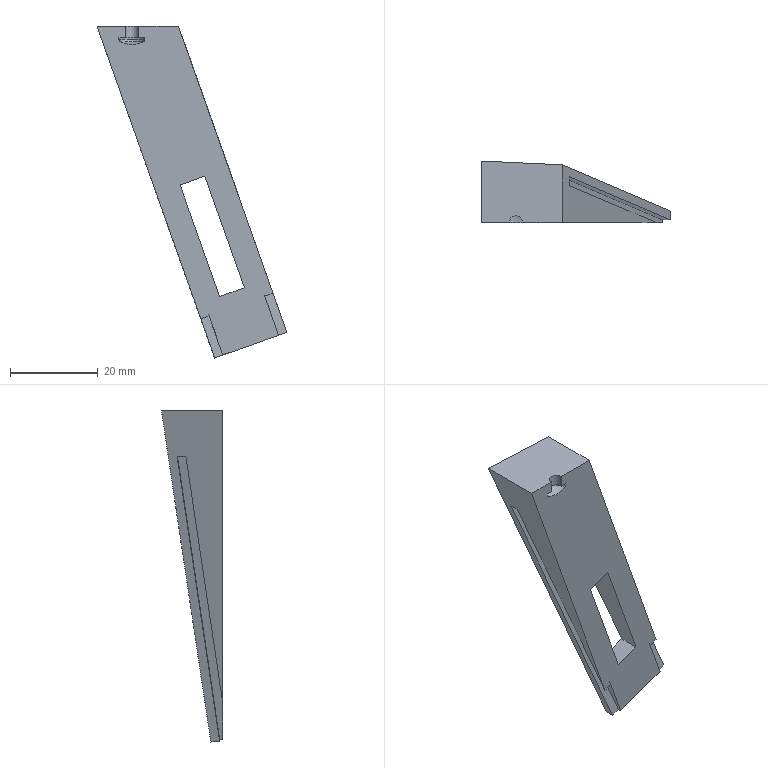Part | STEP file | SLIDE1-LIFTER2_id630_x_t | 1 solid | 23 faces | box 43.318 x 14 x 75.744 mm | volume 9406 mm3 | plane 19 | cylinder 2 | other 2 | commonest cylinder face diameters 3.054 x1 5.904 x1
STEP:
#1=CARTESIAN_POINT('',(-33.767,0.,21.925));
#2=VERTEX_POINT('',#1);
#3=CARTESIAN_POINT('',(-27.862,0.,21.925));
#4=VERTEX_POINT('',#3);
#5=CARTESIAN_POINT('',(-30.814,0.,21.925));
#6=DIRECTION('',(0.,0.,-1.));
#7=DIRECTION('',(-0.9983,0.05901,0.));
#8=AXIS2_PLACEMENT_3D('',#5,#6,#7);
#9=CIRCLE('',#8,2.952);
#10=EDGE_CURVE('',#2,#4,#9,.T.);
#11=ORIENTED_EDGE('',*,*,#10,.T.);
#12=CARTESIAN_POINT('',(-27.862,0.,22.419));
#13=VERTEX_POINT('',#12);
#14=CARTESIAN_POINT('',(-27.862,0.,25.274));
#15=DIRECTION('',(0.,0.,-1.));
#16=VECTOR('',#15,1.);
#17=LINE('',#14,#16);
#18=EDGE_CURVE('',#13,#4,#17,.T.);
#19=ORIENTED_EDGE('',*,*,#18,.F.);
#20=CARTESIAN_POINT('',(-33.767,0.,22.419));
#21=VERTEX_POINT('',#20);
#22=CARTESIAN_POINT('',(-30.814,0.,22.419));
#23=DIRECTION('',(0.,0.,-1.));
#24=DIRECTION('',(-1.,0.,0.));
#25=AXIS2_PLACEMENT_3D('',#22,#23,#24);
#26=CIRCLE('',#25,2.952);
#27=EDGE_CURVE('',#21,#13,#26,.T.);
#28=ORIENTED_EDGE('',*,*,#27,.F.);
#29=CARTESIAN_POINT('',(-33.767,0.,25.274));
#30=DIRECTION('',(0.,0.,1.));
#31=VECTOR('',#30,1.);
#32=LINE('',#29,#31);
#33=EDGE_CURVE('',#2,#21,#32,.T.);
#34=ORIENTED_EDGE('',*,*,#33,.F.);
#35=EDGE_LOOP('',(#11,#19,#28,#34));
#36=FACE_OUTER_BOUND('',#35,.T.);
#37=CARTESIAN_POINT('',(-30.814,0.,25.274));
#38=DIRECTION('',(0.,0.,-1.));
#39=DIRECTION('',(-1.,0.,0.));
#40=AXIS2_PLACEMENT_3D('',#37,#38,#39);
#41=CYLINDRICAL_SURFACE('',#40,2.952);
#42=ADVANCED_FACE('',(#36),#41,.F.);
#43=CARTESIAN_POINT('',(-33.466,0.,21.46));
#44=VERTEX_POINT('',#43);
#45=CARTESIAN_POINT('',(-33.466,0.,21.46));
#46=CARTESIAN_POINT('',(-33.518,0.,21.484));
#47=CARTESIAN_POINT('',(-33.567,0.,21.516));
#48=CARTESIAN_POINT('',(-33.608,0.,21.555));
#49=CARTESIAN_POINT('',(-33.649,0.,21.595));
#50=CARTESIAN_POINT('',(-33.685,0.,21.642));
#51=CARTESIAN_POINT('',(-33.711,0.,21.692));
#52=CARTESIAN_POINT('',(-33.737,0.,21.743));
#53=CARTESIAN_POINT('',(-33.754,0.,21.799));
#54=CARTESIAN_POINT('',(-33.762,0.,21.855));
#55=CARTESIAN_POINT('',(-33.765,0.,21.878));
#56=CARTESIAN_POINT('',(-33.767,0.,21.901));
#57=CARTESIAN_POINT('',(-33.767,0.,21.925));
#58=B_SPLINE_CURVE_WITH_KNOTS('',3,(#45,#46,#47,#48,#49,#50,#51,#52,#53,#54,#55,#56,#57),.UNSPECIFIED.,.F.,.F.,(4,3,3,3,4),(0.,0.294,0.588,0.882,1.),.UNSPECIFIED.);
#59=EDGE_CURVE('',#44,#2,#58,.T.);
#60=ORIENTED_EDGE('',*,*,#59,.F.);
#61=CARTESIAN_POINT('',(-33.458,0.2056,21.46));
#62=VERTEX_POINT('',#61);
#63=CARTESIAN_POINT('',(-33.466,0.,21.46));
#64=CARTESIAN_POINT('',(-33.466,0.06861,21.46));
#65=CARTESIAN_POINT('',(-33.464,0.1372,21.46));
#66=CARTESIAN_POINT('',(-33.458,0.2056,21.46));
#67=B_SPLINE_CURVE_WITH_KNOTS('',3,(#63,#64,#65,#66),.UNSPECIFIED.,.F.,.F.,(4,4),(0.,1.),.UNSPECIFIED.);
#68=EDGE_CURVE('',#44,#62,#67,.T.);
#69=ORIENTED_EDGE('',*,*,#68,.T.);
#70=CARTESIAN_POINT('',(-28.163,0.,21.46));
#71=VERTEX_POINT('',#70);
#72=CARTESIAN_POINT('',(-33.458,0.2056,21.46));
#73=CARTESIAN_POINT('',(-33.406,0.8807,21.46));
#74=CARTESIAN_POINT('',(-33.083,1.531,21.46));
#75=CARTESIAN_POINT('',(-32.071,2.431,21.46));
#76=CARTESIAN_POINT('',(-31.388,2.676,21.46));
#77=CARTESIAN_POINT('',(-30.035,2.624,21.46));
#78=CARTESIAN_POINT('',(-29.373,2.326,21.46));
#79=CARTESIAN_POINT('',(-28.434,1.35,21.46));
#80=CARTESIAN_POINT('',(-28.163,0.6771,21.46));
#81=CARTESIAN_POINT('',(-28.163,0.,21.46));
#82=B_SPLINE_CURVE_WITH_KNOTS('',3,(#72,#73,#74,#75,#76,#77,#78,#79,#80,#81),.UNSPECIFIED.,.F.,.F.,(4,2,2,2,4),(0.,0.25,0.5,0.75,1.),.UNSPECIFIED.);
#83=EDGE_CURVE('',#62,#71,#82,.T.);
#84=ORIENTED_EDGE('',*,*,#83,.T.);
#85=CARTESIAN_POINT('',(-27.862,0.,21.925));
#86=CARTESIAN_POINT('',(-27.862,0.,21.868));
#87=CARTESIAN_POINT('',(-27.872,0.,21.81));
#88=CARTESIAN_POINT('',(-27.891,0.,21.756));
#89=CARTESIAN_POINT('',(-27.91,0.,21.702));
#90=CARTESIAN_POINT('',(-27.938,0.,21.651));
#91=CARTESIAN_POINT('',(-27.974,0.,21.607));
#92=CARTESIAN_POINT('',(-28.009,0.,21.562));
#93=CARTESIAN_POINT('',(-28.053,0.,21.523));
#94=CARTESIAN_POINT('',(-28.101,0.,21.493));
#95=CARTESIAN_POINT('',(-28.121,0.,21.481));
#96=CARTESIAN_POINT('',(-28.142,0.,21.47));
#97=CARTESIAN_POINT('',(-28.163,0.,21.46));
#98=B_SPLINE_CURVE_WITH_KNOTS('',3,(#85,#86,#87,#88,#89,#90,#91,#92,#93,#94,#95,#96,#97),.UNSPECIFIED.,.F.,.F.,(4,3,3,3,4),(0.,0.294,0.588,0.882,1.),.UNSPECIFIED.);
#99=EDGE_CURVE('',#4,#71,#98,.T.);
#100=ORIENTED_EDGE('',*,*,#99,.F.);
#101=ORIENTED_EDGE('',*,*,#10,.F.);
#102=EDGE_LOOP('',(#60,#69,#84,#100,#101));
#103=FACE_OUTER_BOUND('',#102,.T.);
#104=CARTESIAN_POINT('',(-33.253,0.1442,21.925));
#105=DIRECTION('',(-0.05901,-0.9983,0.));
#106=DIRECTION('',(-0.9983,0.05901,0.));
#107=AXIS2_PLACEMENT_3D('',#104,#105,#106);
#108=CIRCLE('',#107,0.509);
#109=CARTESIAN_POINT('',(-30.814,0.,21.925));
#110=DIRECTION('',(0.,0.,1.));
#111=AXIS1_PLACEMENT('',#109,#110);
#112=SURFACE_OF_REVOLUTION('',#108,#111);
#113=ADVANCED_FACE('',(#103),#112,.T.);
#114=CARTESIAN_POINT('',(-29.287,0.,22.419));
#115=VERTEX_POINT('',#114);
#116=CARTESIAN_POINT('',(-32.341,0.,22.419));
#117=VERTEX_POINT('',#116);
#118=CARTESIAN_POINT('',(-30.814,0.,22.419));
#119=DIRECTION('',(0.,0.,1.));
#120=DIRECTION('',(1.,0.,0.));
#121=AXIS2_PLACEMENT_3D('',#118,#119,#120);
#122=CIRCLE('',#121,1.527);
#123=EDGE_CURVE('',#115,#117,#122,.T.);
#124=ORIENTED_EDGE('',*,*,#123,.T.);
#125=CARTESIAN_POINT('',(-30.814,0.,22.419));
#126=DIRECTION('',(-1.,0.,0.));
#127=VECTOR('',#126,1.);
#128=LINE('',#125,#127);
#129=EDGE_CURVE('',#117,#21,#128,.T.);
#130=ORIENTED_EDGE('',*,*,#129,.T.);
#131=ORIENTED_EDGE('',*,*,#27,.T.);
#132=CARTESIAN_POINT('',(-30.814,0.,22.419));
#133=DIRECTION('',(-1.,0.,0.));
#134=VECTOR('',#133,1.);
#135=LINE('',#132,#134);
#136=EDGE_CURVE('',#13,#115,#135,.T.);
#137=ORIENTED_EDGE('',*,*,#136,.T.);
#138=EDGE_LOOP('',(#124,#130,#131,#137));
#139=FACE_OUTER_BOUND('',#138,.T.);
#140=CARTESIAN_POINT('',(-30.814,0.,22.419));
#141=DIRECTION('',(0.,0.,-1.));
#142=DIRECTION('',(-1.,0.,0.));
#143=AXIS2_PLACEMENT_3D('',#140,#141,#142);
#144=PLANE('',#143);
#145=ADVANCED_FACE('',(#139),#144,.T.);
#146=ORIENTED_EDGE('',*,*,#68,.F.);
#147=CARTESIAN_POINT('',(-30.814,0.,20.892));
#148=VERTEX_POINT('',#147);
#149=CARTESIAN_POINT('',(-30.814,0.,27.364));
#150=DIRECTION('',(0.,1.,0.));
#151=DIRECTION('',(0.,0.,-1.));
#152=AXIS2_PLACEMENT_3D('',#149,#150,#151);
#153=CIRCLE('',#152,6.472);
#154=EDGE_CURVE('',#148,#44,#153,.T.);
#155=ORIENTED_EDGE('',*,*,#154,.F.);
#156=CARTESIAN_POINT('',(-28.163,0.,21.46));
#157=CARTESIAN_POINT('',(-29.,0.,21.084));
#158=CARTESIAN_POINT('',(-29.91,0.,20.892));
#159=CARTESIAN_POINT('',(-30.814,0.,20.892));
#160=B_SPLINE_CURVE_WITH_KNOTS('',3,(#156,#157,#158,#159),.UNSPECIFIED.,.F.,.F.,(4,4),(0.,1.),.UNSPECIFIED.);
#161=EDGE_CURVE('',#71,#148,#160,.T.);
#162=ORIENTED_EDGE('',*,*,#161,.F.);
#163=ORIENTED_EDGE('',*,*,#83,.F.);
#164=EDGE_LOOP('',(#146,#155,#162,#163));
#165=FACE_OUTER_BOUND('',#164,.T.);
#166=CARTESIAN_POINT('',(-30.814,0.,20.892));
#167=CARTESIAN_POINT('',(-30.814,-0.9232,20.892));
#168=CARTESIAN_POINT('',(-30.814,-1.826,21.087));
#169=CARTESIAN_POINT('',(-30.814,-2.667,21.467));
#170=(BOUNDED_CURVE()B_SPLINE_CURVE(3,(#166,#167,#168,#169),.UNSPECIFIED.,.F.,.F.)B_SPLINE_CURVE_WITH_KNOTS((4,4),(0.,1.),.UNSPECIFIED.)CURVE()GEOMETRIC_REPRESENTATION_ITEM()RATIONAL_B_SPLINE_CURVE((1.,0.985,0.985,1.))REPRESENTATION_ITEM(''));
#171=CARTESIAN_POINT('',(-30.814,0.,27.364));
#172=DIRECTION('',(0.,0.,-1.));
#173=AXIS1_PLACEMENT('',#171,#172);
#174=SURFACE_OF_REVOLUTION('',#170,#173);
#175=ADVANCED_FACE('',(#165),#174,.T.);
#176=CARTESIAN_POINT('',(-33.148,10.407,15.179));
#177=VERTEX_POINT('',#176);
#178=CARTESIAN_POINT('',(-33.148,8.387,15.179));
#179=VERTEX_POINT('',#178);
#180=CARTESIAN_POINT('',(-33.148,10.407,15.179));
#181=DIRECTION('',(0.,-1.,0.));
#182=VECTOR('',#181,1.);
#183=LINE('',#180,#182);
#184=EDGE_CURVE('',#177,#179,#183,.T.);
#185=ORIENTED_EDGE('',*,*,#184,.F.);
#186=CARTESIAN_POINT('',(-10.063,0.6875,-50.01));
#187=VERTEX_POINT('',#186);
#188=CARTESIAN_POINT('',(-10.063,0.6875,-50.01));
#189=DIRECTION('',(-0.3306,0.1392,0.9335));
#190=VECTOR('',#189,1.);
#191=LINE('',#188,#190);
#192=EDGE_CURVE('',#187,#177,#191,.T.);
#193=ORIENTED_EDGE('',*,*,#192,.F.);
#194=CARTESIAN_POINT('',(-10.063,0.,-50.01));
#195=VERTEX_POINT('',#194);
#196=CARTESIAN_POINT('',(-10.063,0.,-50.01));
#197=DIRECTION('',(0.,1.,0.));
#198=VECTOR('',#197,1.);
#199=LINE('',#196,#198);
#200=EDGE_CURVE('',#195,#187,#199,.T.);
#201=ORIENTED_EDGE('',*,*,#200,.F.);
#202=CARTESIAN_POINT('',(-13.227,0.,-41.075));
#203=VERTEX_POINT('',#202);
#204=CARTESIAN_POINT('',(-13.227,0.,-41.075));
#205=DIRECTION('',(0.3338,0.,-0.9426));
#206=VECTOR('',#205,1.);
#207=LINE('',#204,#206);
#208=EDGE_CURVE('',#203,#195,#207,.T.);
#209=ORIENTED_EDGE('',*,*,#208,.F.);
#210=CARTESIAN_POINT('',(-33.148,8.387,15.179));
#211=DIRECTION('',(0.3306,-0.1392,-0.9335));
#212=VECTOR('',#211,1.);
#213=LINE('',#210,#212);
#214=EDGE_CURVE('',#179,#203,#213,.T.);
#215=ORIENTED_EDGE('',*,*,#214,.F.);
#216=EDGE_LOOP('',(#185,#193,#201,#209,#215));
#217=FACE_OUTER_BOUND('',#216,.T.);
#218=CARTESIAN_POINT('',(-36.517,0.,24.692));
#219=DIRECTION('',(0.9426,0.,0.3338));
#220=DIRECTION('',(0.3338,0.,-0.9426));
#221=AXIS2_PLACEMENT_3D('',#218,#219,#220);
#222=PLANE('',#221);
#223=ADVANCED_FACE('',(#217),#222,.F.);
#224=CARTESIAN_POINT('',(-20.422,10.407,19.685));
#225=VERTEX_POINT('',#224);
#226=CARTESIAN_POINT('',(2.662,0.6875,-45.504));
#227=VERTEX_POINT('',#226);
#228=CARTESIAN_POINT('',(-20.422,10.407,19.685));
#229=DIRECTION('',(0.3306,-0.1392,-0.9335));
#230=VECTOR('',#229,1.);
#231=LINE('',#228,#230);
#232=EDGE_CURVE('',#225,#227,#231,.T.);
#233=ORIENTED_EDGE('',*,*,#232,.F.);
#234=CARTESIAN_POINT('',(-20.422,8.387,19.685));
#235=VERTEX_POINT('',#234);
#236=CARTESIAN_POINT('',(-20.422,8.387,19.685));
#237=DIRECTION('',(0.,1.,0.));
#238=VECTOR('',#237,1.);
#239=LINE('',#236,#238);
#240=EDGE_CURVE('',#235,#225,#239,.T.);
#241=ORIENTED_EDGE('',*,*,#240,.F.);
#242=CARTESIAN_POINT('',(-0.5016,0.,-36.569));
#243=VERTEX_POINT('',#242);
#244=CARTESIAN_POINT('',(-0.5016,0.,-36.569));
#245=DIRECTION('',(-0.3306,0.1392,0.9335));
#246=VECTOR('',#245,1.);
#247=LINE('',#244,#246);
#248=EDGE_CURVE('',#243,#235,#247,.T.);
#249=ORIENTED_EDGE('',*,*,#248,.F.);
#250=CARTESIAN_POINT('',(2.662,0.,-45.504));
#251=VERTEX_POINT('',#250);
#252=CARTESIAN_POINT('',(2.662,0.,-45.504));
#253=DIRECTION('',(-0.3338,0.,0.9426));
#254=VECTOR('',#253,1.);
#255=LINE('',#252,#254);
#256=EDGE_CURVE('',#251,#243,#255,.T.);
#257=ORIENTED_EDGE('',*,*,#256,.F.);
#258=CARTESIAN_POINT('',(2.662,0.,-45.504));
#259=DIRECTION('',(0.,-1.,0.));
#260=VECTOR('',#259,1.);
#261=LINE('',#258,#260);
#262=EDGE_CURVE('',#227,#251,#261,.T.);
#263=ORIENTED_EDGE('',*,*,#262,.F.);
#264=EDGE_LOOP('',(#233,#241,#249,#257,#263));
#265=FACE_OUTER_BOUND('',#264,.T.);
#266=CARTESIAN_POINT('',(-23.791,0.,29.199));
#267=DIRECTION('',(-0.9426,0.,-0.3338));
#268=DIRECTION('',(-0.3338,0.,0.9426));
#269=AXIS2_PLACEMENT_3D('',#266,#267,#268);
#270=PLANE('',#269);
#271=ADVANCED_FACE('',(#265),#270,.F.);
#272=CARTESIAN_POINT('',(-18.537,10.407,20.353));
#273=VERTEX_POINT('',#272);
#274=CARTESIAN_POINT('',(-18.537,10.407,20.353));
#275=DIRECTION('',(-0.9426,0.,-0.3338));
#276=VECTOR('',#275,1.);
#277=LINE('',#274,#276);
#278=EDGE_CURVE('',#273,#225,#277,.T.);
#279=ORIENTED_EDGE('',*,*,#278,.F.);
#280=CARTESIAN_POINT('',(-18.537,8.387,20.353));
#281=VERTEX_POINT('',#280);
#282=CARTESIAN_POINT('',(-18.537,0.,20.353));
#283=DIRECTION('',(0.,-1.,0.));
#284=VECTOR('',#283,1.);
#285=LINE('',#282,#284);
#286=EDGE_CURVE('',#273,#281,#285,.T.);
#287=ORIENTED_EDGE('',*,*,#286,.T.);
#288=CARTESIAN_POINT('',(-20.422,8.387,19.685));
#289=DIRECTION('',(0.9426,0.,0.3338));
#290=VECTOR('',#289,1.);
#291=LINE('',#288,#290);
#292=EDGE_CURVE('',#235,#281,#291,.T.);
#293=ORIENTED_EDGE('',*,*,#292,.F.);
#294=ORIENTED_EDGE('',*,*,#240,.T.);
#295=EDGE_LOOP('',(#279,#287,#293,#294));
#296=FACE_OUTER_BOUND('',#295,.T.);
#297=CARTESIAN_POINT('',(-18.537,8.387,20.353));
#298=DIRECTION('',(0.3338,0.,-0.9426));
#299=DIRECTION('',(-0.9426,0.,-0.3338));
#300=AXIS2_PLACEMENT_3D('',#297,#298,#299);
#301=PLANE('',#300);
#302=ADVANCED_FACE('',(#296),#301,.T.);
#303=CARTESIAN_POINT('',(1.384,0.,-35.901));
#304=VERTEX_POINT('',#303);
#305=CARTESIAN_POINT('',(-18.537,8.387,20.353));
#306=DIRECTION('',(0.3306,-0.1392,-0.9335));
#307=VECTOR('',#306,1.);
#308=LINE('',#305,#307);
#309=EDGE_CURVE('',#281,#304,#308,.T.);
#310=ORIENTED_EDGE('',*,*,#309,.T.);
#311=CARTESIAN_POINT('',(-0.5016,0.,-36.569));
#312=DIRECTION('',(0.9426,0.,0.3338));
#313=VECTOR('',#312,1.);
#314=LINE('',#311,#313);
#315=EDGE_CURVE('',#243,#304,#314,.T.);
#316=ORIENTED_EDGE('',*,*,#315,.F.);
#317=ORIENTED_EDGE('',*,*,#248,.T.);
#318=ORIENTED_EDGE('',*,*,#292,.T.);
#319=EDGE_LOOP('',(#310,#316,#317,#318));
#320=FACE_OUTER_BOUND('',#319,.T.);
#321=CARTESIAN_POINT('',(1.384,0.,-35.901));
#322=DIRECTION('',(0.04646,0.9903,-0.1312));
#323=DIRECTION('',(0.,0.1313,0.9913));
#324=AXIS2_PLACEMENT_3D('',#321,#322,#323);
#325=PLANE('',#324);
#326=ADVANCED_FACE('',(#320),#325,.T.);
#327=ORIENTED_EDGE('',*,*,#232,.T.);
#328=CARTESIAN_POINT('',(4.548,0.6875,-44.836));
#329=VERTEX_POINT('',#328);
#330=CARTESIAN_POINT('',(-11.949,0.6875,-50.678));
#331=DIRECTION('',(0.9426,0.,0.3338));
#332=VECTOR('',#331,1.);
#333=LINE('',#330,#332);
#334=EDGE_CURVE('',#227,#329,#333,.T.);
#335=ORIENTED_EDGE('',*,*,#334,.T.);
#336=CARTESIAN_POINT('',(4.548,0.6875,-44.836));
#337=DIRECTION('',(-0.3306,0.1392,0.9335));
#338=VECTOR('',#337,1.);
#339=LINE('',#336,#338);
#340=EDGE_CURVE('',#329,#273,#339,.T.);
#341=ORIENTED_EDGE('',*,*,#340,.T.);
#342=ORIENTED_EDGE('',*,*,#278,.T.);
#343=EDGE_LOOP('',(#327,#335,#341,#342));
#344=FACE_OUTER_BOUND('',#343,.T.);
#345=CARTESIAN_POINT('',(-18.537,10.407,20.353));
#346=DIRECTION('',(-0.04646,-0.9903,0.1312));
#347=DIRECTION('',(0.,-0.1313,-0.9913));
#348=AXIS2_PLACEMENT_3D('',#345,#346,#347);
#349=PLANE('',#348);
#350=ADVANCED_FACE('',(#344),#349,.T.);
#351=ORIENTED_EDGE('',*,*,#214,.T.);
#352=CARTESIAN_POINT('',(-15.113,0.,-41.743));
#353=VERTEX_POINT('',#352);
#354=CARTESIAN_POINT('',(-15.113,0.,-41.743));
#355=DIRECTION('',(0.9426,0.,0.3338));
#356=VECTOR('',#355,1.);
#357=LINE('',#354,#356);
#358=EDGE_CURVE('',#353,#203,#357,.T.);
#359=ORIENTED_EDGE('',*,*,#358,.F.);
#360=CARTESIAN_POINT('',(-35.033,8.387,14.511));
#361=VERTEX_POINT('',#360);
#362=CARTESIAN_POINT('',(-15.113,0.,-41.743));
#363=DIRECTION('',(-0.3306,0.1392,0.9335));
#364=VECTOR('',#363,1.);
#365=LINE('',#362,#364);
#366=EDGE_CURVE('',#353,#361,#365,.T.);
#367=ORIENTED_EDGE('',*,*,#366,.T.);
#368=CARTESIAN_POINT('',(-35.033,8.387,14.511));
#369=DIRECTION('',(-0.9426,0.,-0.3338));
#370=VECTOR('',#369,1.);
#371=LINE('',#368,#370);
#372=EDGE_CURVE('',#179,#361,#371,.T.);
#373=ORIENTED_EDGE('',*,*,#372,.F.);
#374=EDGE_LOOP('',(#351,#359,#367,#373));
#375=FACE_OUTER_BOUND('',#374,.T.);
#376=CARTESIAN_POINT('',(-35.033,8.387,14.511));
#377=DIRECTION('',(0.04646,0.9903,-0.1312));
#378=DIRECTION('',(0.,0.1313,0.9913));
#379=AXIS2_PLACEMENT_3D('',#376,#377,#378);
#380=PLANE('',#379);
#381=ADVANCED_FACE('',(#375),#380,.T.);
#382=ORIENTED_EDGE('',*,*,#372,.T.);
#383=CARTESIAN_POINT('',(-35.033,10.407,14.511));
#384=VERTEX_POINT('',#383);
#385=CARTESIAN_POINT('',(-35.033,0.,14.511));
#386=DIRECTION('',(0.,1.,0.));
#387=VECTOR('',#386,1.);
#388=LINE('',#385,#387);
#389=EDGE_CURVE('',#361,#384,#388,.T.);
#390=ORIENTED_EDGE('',*,*,#389,.T.);
#391=CARTESIAN_POINT('',(-33.148,10.407,15.179));
#392=DIRECTION('',(-0.9426,0.,-0.3338));
#393=VECTOR('',#392,1.);
#394=LINE('',#391,#393);
#395=EDGE_CURVE('',#177,#384,#394,.T.);
#396=ORIENTED_EDGE('',*,*,#395,.F.);
#397=ORIENTED_EDGE('',*,*,#184,.T.);
#398=EDGE_LOOP('',(#382,#390,#396,#397));
#399=FACE_OUTER_BOUND('',#398,.T.);
#400=CARTESIAN_POINT('',(-35.033,10.407,14.511));
#401=DIRECTION('',(0.3338,0.,-0.9426));
#402=DIRECTION('',(-0.9426,0.,-0.3338));
#403=AXIS2_PLACEMENT_3D('',#400,#401,#402);
#404=PLANE('',#403);
#405=ADVANCED_FACE('',(#399),#404,.T.);
#406=ORIENTED_EDGE('',*,*,#395,.T.);
#407=CARTESIAN_POINT('',(-11.949,0.6875,-50.678));
#408=VERTEX_POINT('',#407);
#409=CARTESIAN_POINT('',(-35.033,10.407,14.511));
#410=DIRECTION('',(0.3306,-0.1392,-0.9335));
#411=VECTOR('',#410,1.);
#412=LINE('',#409,#411);
#413=EDGE_CURVE('',#384,#408,#412,.T.);
#414=ORIENTED_EDGE('',*,*,#413,.T.);
#415=CARTESIAN_POINT('',(-11.949,0.6875,-50.678));
#416=DIRECTION('',(0.9426,0.,0.3338));
#417=VECTOR('',#416,1.);
#418=LINE('',#415,#417);
#419=EDGE_CURVE('',#408,#187,#418,.T.);
#420=ORIENTED_EDGE('',*,*,#419,.T.);
#421=ORIENTED_EDGE('',*,*,#192,.T.);
#422=EDGE_LOOP('',(#406,#414,#420,#421));
#423=FACE_OUTER_BOUND('',#422,.T.);
#424=CARTESIAN_POINT('',(-11.328,0.4262,-52.431));
#425=DIRECTION('',(-0.04646,-0.9903,0.1312));
#426=DIRECTION('',(0.,-0.1313,-0.9913));
#427=AXIS2_PLACEMENT_3D('',#424,#425,#426);
#428=PLANE('',#427);
#429=ADVANCED_FACE('',(#423),#428,.T.);
#430=CARTESIAN_POINT('',(-29.287,0.,25.066));
#431=VERTEX_POINT('',#430);
#432=CARTESIAN_POINT('',(-32.341,0.,25.066));
#433=VERTEX_POINT('',#432);
#434=CARTESIAN_POINT('',(-30.814,0.,25.066));
#435=DIRECTION('',(0.,0.,1.));
#436=DIRECTION('',(1.,0.,0.));
#437=AXIS2_PLACEMENT_3D('',#434,#435,#436);
#438=CIRCLE('',#437,1.527);
#439=EDGE_CURVE('',#431,#433,#438,.T.);
#440=ORIENTED_EDGE('',*,*,#439,.T.);
#441=CARTESIAN_POINT('',(-32.341,0.,27.));
#442=DIRECTION('',(0.,0.,1.));
#443=VECTOR('',#442,1.);
#444=LINE('',#441,#443);
#445=EDGE_CURVE('',#117,#433,#444,.T.);
#446=ORIENTED_EDGE('',*,*,#445,.F.);
#447=ORIENTED_EDGE('',*,*,#123,.F.);
#448=CARTESIAN_POINT('',(-29.287,0.,27.));
#449=DIRECTION('',(0.,0.,-1.));
#450=VECTOR('',#449,1.);
#451=LINE('',#448,#450);
#452=EDGE_CURVE('',#431,#115,#451,.T.);
#453=ORIENTED_EDGE('',*,*,#452,.F.);
#454=EDGE_LOOP('',(#440,#446,#447,#453));
#455=FACE_OUTER_BOUND('',#454,.T.);
#456=CARTESIAN_POINT('',(-30.814,0.,25.274));
#457=DIRECTION('',(0.,0.,1.));
#458=DIRECTION('',(1.,0.,0.));
#459=AXIS2_PLACEMENT_3D('',#456,#457,#458);
#460=CYLINDRICAL_SURFACE('',#459,1.527);
#461=ADVANCED_FACE('',(#455),#460,.F.);
#462=CARTESIAN_POINT('',(-19.831,0.,-11.194));
#463=VERTEX_POINT('',#462);
#464=CARTESIAN_POINT('',(-10.818,0.,-36.645));
#465=VERTEX_POINT('',#464);
#466=CARTESIAN_POINT('',(-10.818,0.,-36.645));
#467=DIRECTION('',(0.3338,0.,-0.9426));
#468=VECTOR('',#467,1.);
#469=LINE('',#466,#468);
#470=EDGE_CURVE('',#463,#465,#469,.T.);
#471=ORIENTED_EDGE('',*,*,#470,.F.);
#472=CARTESIAN_POINT('',(-14.175,0.,-9.191));
#473=VERTEX_POINT('',#472);
#474=CARTESIAN_POINT('',(-19.831,0.,-11.194));
#475=DIRECTION('',(-0.9426,0.,-0.3338));
#476=VECTOR('',#475,1.);
#477=LINE('',#474,#476);
#478=EDGE_CURVE('',#473,#463,#477,.T.);
#479=ORIENTED_EDGE('',*,*,#478,.F.);
#480=CARTESIAN_POINT('',(-5.162,0.,-34.643));
#481=VERTEX_POINT('',#480);
#482=CARTESIAN_POINT('',(-14.175,0.,-9.191));
#483=DIRECTION('',(-0.3338,0.,0.9426));
#484=VECTOR('',#483,1.);
#485=LINE('',#482,#484);
#486=EDGE_CURVE('',#481,#473,#485,.T.);
#487=ORIENTED_EDGE('',*,*,#486,.F.);
#488=CARTESIAN_POINT('',(-5.162,0.,-34.643));
#489=DIRECTION('',(0.9426,0.,0.3338));
#490=VECTOR('',#489,1.);
#491=LINE('',#488,#490);
#492=EDGE_CURVE('',#465,#481,#491,.T.);
#493=ORIENTED_EDGE('',*,*,#492,.F.);
#494=EDGE_LOOP('',(#471,#479,#487,#493));
#495=FACE_BOUND('',#494,.T.);
#496=CARTESIAN_POINT('',(-11.949,0.,-50.678));
#497=DIRECTION('',(0.9426,0.,0.3338));
#498=VECTOR('',#497,1.);
#499=LINE('',#496,#498);
#500=EDGE_CURVE('',#195,#251,#499,.T.);
#501=ORIENTED_EDGE('',*,*,#500,.T.);
#502=ORIENTED_EDGE('',*,*,#256,.T.);
#503=ORIENTED_EDGE('',*,*,#315,.T.);
#504=CARTESIAN_POINT('',(-20.206,0.,25.066));
#505=VERTEX_POINT('',#504);
#506=CARTESIAN_POINT('',(4.548,0.,-44.836));
#507=DIRECTION('',(-0.3338,0.,0.9426));
#508=VECTOR('',#507,1.);
#509=LINE('',#506,#508);
#510=EDGE_CURVE('',#304,#505,#509,.T.);
#511=ORIENTED_EDGE('',*,*,#510,.T.);
#512=CARTESIAN_POINT('',(-20.206,0.,25.066));
#513=DIRECTION('',(-1.,0.,0.));
#514=VECTOR('',#513,1.);
#515=LINE('',#512,#514);
#516=EDGE_CURVE('',#505,#431,#515,.T.);
#517=ORIENTED_EDGE('',*,*,#516,.T.);
#518=ORIENTED_EDGE('',*,*,#452,.T.);
#519=ORIENTED_EDGE('',*,*,#136,.F.);
#520=ORIENTED_EDGE('',*,*,#18,.T.);
#521=ORIENTED_EDGE('',*,*,#99,.T.);
#522=ORIENTED_EDGE('',*,*,#161,.T.);
#523=ORIENTED_EDGE('',*,*,#154,.T.);
#524=ORIENTED_EDGE('',*,*,#59,.T.);
#525=ORIENTED_EDGE('',*,*,#33,.T.);
#526=ORIENTED_EDGE('',*,*,#129,.F.);
#527=ORIENTED_EDGE('',*,*,#445,.T.);
#528=CARTESIAN_POINT('',(-38.771,0.,25.066));
#529=VERTEX_POINT('',#528);
#530=CARTESIAN_POINT('',(-20.206,0.,25.066));
#531=DIRECTION('',(-1.,0.,0.));
#532=VECTOR('',#531,1.);
#533=LINE('',#530,#532);
#534=EDGE_CURVE('',#433,#529,#533,.T.);
#535=ORIENTED_EDGE('',*,*,#534,.T.);
#536=CARTESIAN_POINT('',(-38.771,0.,25.066));
#537=DIRECTION('',(0.3338,0.,-0.9426));
#538=VECTOR('',#537,1.);
#539=LINE('',#536,#538);
#540=EDGE_CURVE('',#529,#353,#539,.T.);
#541=ORIENTED_EDGE('',*,*,#540,.T.);
#542=ORIENTED_EDGE('',*,*,#358,.T.);
#543=ORIENTED_EDGE('',*,*,#208,.T.);
#544=EDGE_LOOP('',(#501,#502,#503,#511,#517,#518,#519,#520,#521,#522,#523,#524,#525,#526,#527,#535,#541,#542,#543));
#545=FACE_BOUND('',#544,.T.);
#546=CARTESIAN_POINT('',(-30.,0.,27.));
#547=DIRECTION('',(0.,-1.,0.));
#548=DIRECTION('',(0.,0.,-1.));
#549=AXIS2_PLACEMENT_3D('',#546,#547,#548);
#550=PLANE('',#549);
#551=ADVANCED_FACE('',(#495,#545),#550,.T.);
#552=CARTESIAN_POINT('',(-20.206,13.129,25.066));
#553=VERTEX_POINT('',#552);
#554=CARTESIAN_POINT('',(4.548,2.707,-44.836));
#555=VERTEX_POINT('',#554);
#556=CARTESIAN_POINT('',(-20.206,13.129,25.066));
#557=DIRECTION('',(0.3306,-0.1392,-0.9335));
#558=VECTOR('',#557,1.);
#559=LINE('',#556,#558);
#560=EDGE_CURVE('',#553,#555,#559,.T.);
#561=ORIENTED_EDGE('',*,*,#560,.F.);
#562=CARTESIAN_POINT('',(-20.206,0.,25.066));
#563=DIRECTION('',(0.,-1.,0.));
#564=VECTOR('',#563,1.);
#565=LINE('',#562,#564);
#566=EDGE_CURVE('',#553,#505,#565,.T.);
#567=ORIENTED_EDGE('',*,*,#566,.T.);
#568=ORIENTED_EDGE('',*,*,#510,.F.);
#569=ORIENTED_EDGE('',*,*,#309,.F.);
#570=ORIENTED_EDGE('',*,*,#286,.F.);
#571=ORIENTED_EDGE('',*,*,#340,.F.);
#572=CARTESIAN_POINT('',(4.548,0.,-44.836));
#573=DIRECTION('',(0.,1.,0.));
#574=VECTOR('',#573,1.);
#575=LINE('',#572,#574);
#576=EDGE_CURVE('',#329,#555,#575,.T.);
#577=ORIENTED_EDGE('',*,*,#576,.T.);
#578=EDGE_LOOP('',(#561,#567,#568,#569,#570,#571,#577));
#579=FACE_OUTER_BOUND('',#578,.T.);
#580=CARTESIAN_POINT('',(4.548,0.,-44.836));
#581=DIRECTION('',(-0.9426,0.,-0.3338));
#582=DIRECTION('',(-0.3338,0.,0.9426));
#583=AXIS2_PLACEMENT_3D('',#580,#581,#582);
#584=PLANE('',#583);
#585=ADVANCED_FACE('',(#579),#584,.F.);
#586=ORIENTED_EDGE('',*,*,#200,.T.);
#587=ORIENTED_EDGE('',*,*,#419,.F.);
#588=CARTESIAN_POINT('',(-11.949,2.707,-50.678));
#589=VERTEX_POINT('',#588);
#590=CARTESIAN_POINT('',(-11.949,0.,-50.678));
#591=DIRECTION('',(0.,1.,0.));
#592=VECTOR('',#591,1.);
#593=LINE('',#590,#592);
#594=EDGE_CURVE('',#408,#589,#593,.T.);
#595=ORIENTED_EDGE('',*,*,#594,.T.);
#596=CARTESIAN_POINT('',(4.548,2.707,-44.836));
#597=DIRECTION('',(-0.9426,0.,-0.3338));
#598=VECTOR('',#597,1.);
#599=LINE('',#596,#598);
#600=EDGE_CURVE('',#555,#589,#599,.T.);
#601=ORIENTED_EDGE('',*,*,#600,.F.);
#602=ORIENTED_EDGE('',*,*,#576,.F.);
#603=ORIENTED_EDGE('',*,*,#334,.F.);
#604=ORIENTED_EDGE('',*,*,#262,.T.);
#605=ORIENTED_EDGE('',*,*,#500,.F.);
#606=EDGE_LOOP('',(#586,#587,#595,#601,#602,#603,#604,#605));
#607=FACE_OUTER_BOUND('',#606,.T.);
#608=CARTESIAN_POINT('',(-11.949,0.,-50.678));
#609=DIRECTION('',(-0.3338,0.,0.9426));
#610=DIRECTION('',(0.9426,0.,0.3338));
#611=AXIS2_PLACEMENT_3D('',#608,#609,#610);
#612=PLANE('',#611);
#613=ADVANCED_FACE('',(#607),#612,.F.);
#614=CARTESIAN_POINT('',(-38.771,14.,25.066));
#615=VERTEX_POINT('',#614);
#616=CARTESIAN_POINT('',(-38.771,0.,25.066));
#617=DIRECTION('',(0.,1.,0.));
#618=VECTOR('',#617,1.);
#619=LINE('',#616,#618);
#620=EDGE_CURVE('',#529,#615,#619,.T.);
#621=ORIENTED_EDGE('',*,*,#620,.T.);
#622=CARTESIAN_POINT('',(-11.949,2.707,-50.678));
#623=DIRECTION('',(-0.3306,0.1392,0.9335));
#624=VECTOR('',#623,1.);
#625=LINE('',#622,#624);
#626=EDGE_CURVE('',#589,#615,#625,.T.);
#627=ORIENTED_EDGE('',*,*,#626,.F.);
#628=ORIENTED_EDGE('',*,*,#594,.F.);
#629=ORIENTED_EDGE('',*,*,#413,.F.);
#630=ORIENTED_EDGE('',*,*,#389,.F.);
#631=ORIENTED_EDGE('',*,*,#366,.F.);
#632=ORIENTED_EDGE('',*,*,#540,.F.);
#633=EDGE_LOOP('',(#621,#627,#628,#629,#630,#631,#632));
#634=FACE_OUTER_BOUND('',#633,.T.);
#635=CARTESIAN_POINT('',(-38.771,0.,25.066));
#636=DIRECTION('',(0.9426,0.,0.3338));
#637=DIRECTION('',(0.3338,0.,-0.9426));
#638=AXIS2_PLACEMENT_3D('',#635,#636,#637);
#639=PLANE('',#638);
#640=ADVANCED_FACE('',(#634),#639,.F.);
#641=ORIENTED_EDGE('',*,*,#534,.F.);
#642=ORIENTED_EDGE('',*,*,#439,.F.);
#643=ORIENTED_EDGE('',*,*,#516,.F.);
#644=ORIENTED_EDGE('',*,*,#566,.F.);
#645=CARTESIAN_POINT('',(-38.771,14.,25.066));
#646=DIRECTION('',(0.9989,-0.04686,0.));
#647=VECTOR('',#646,1.);
#648=LINE('',#645,#647);
#649=EDGE_CURVE('',#615,#553,#648,.T.);
#650=ORIENTED_EDGE('',*,*,#649,.F.);
#651=ORIENTED_EDGE('',*,*,#620,.F.);
#652=EDGE_LOOP('',(#641,#642,#643,#644,#650,#651));
#653=FACE_OUTER_BOUND('',#652,.T.);
#654=CARTESIAN_POINT('',(-20.206,0.,25.066));
#655=DIRECTION('',(0.,0.,-1.));
#656=DIRECTION('',(-1.,0.,0.));
#657=AXIS2_PLACEMENT_3D('',#654,#655,#656);
#658=PLANE('',#657);
#659=ADVANCED_FACE('',(#653),#658,.F.);
#660=CARTESIAN_POINT('',(-19.831,8.308,-11.194));
#661=VERTEX_POINT('',#660);
#662=CARTESIAN_POINT('',(-19.831,0.,-11.194));
#663=DIRECTION('',(0.,1.,0.));
#664=VECTOR('',#663,1.);
#665=LINE('',#662,#664);
#666=EDGE_CURVE('',#463,#661,#665,.T.);
#667=ORIENTED_EDGE('',*,*,#666,.F.);
#668=ORIENTED_EDGE('',*,*,#470,.T.);
#669=CARTESIAN_POINT('',(-10.818,4.513,-36.645));
#670=VERTEX_POINT('',#669);
#671=CARTESIAN_POINT('',(-10.818,0.,-36.645));
#672=DIRECTION('',(0.,-1.,0.));
#673=VECTOR('',#672,1.);
#674=LINE('',#671,#673);
#675=EDGE_CURVE('',#670,#465,#674,.T.);
#676=ORIENTED_EDGE('',*,*,#675,.F.);
#677=CARTESIAN_POINT('',(-19.831,8.308,-11.194));
#678=DIRECTION('',(0.3306,-0.1392,-0.9335));
#679=VECTOR('',#678,1.);
#680=LINE('',#677,#679);
#681=EDGE_CURVE('',#661,#670,#680,.T.);
#682=ORIENTED_EDGE('',*,*,#681,.F.);
#683=EDGE_LOOP('',(#667,#668,#676,#682));
#684=FACE_OUTER_BOUND('',#683,.T.);
#685=CARTESIAN_POINT('',(-10.818,0.,-36.645));
#686=DIRECTION('',(0.9426,0.,0.3338));
#687=DIRECTION('',(0.3338,0.,-0.9426));
#688=AXIS2_PLACEMENT_3D('',#685,#686,#687);
#689=PLANE('',#688);
#690=ADVANCED_FACE('',(#684),#689,.T.);
#691=ORIENTED_EDGE('',*,*,#675,.T.);
#692=ORIENTED_EDGE('',*,*,#492,.T.);
#693=CARTESIAN_POINT('',(-5.162,4.513,-34.643));
#694=VERTEX_POINT('',#693);
#695=CARTESIAN_POINT('',(-5.162,0.,-34.643));
#696=DIRECTION('',(0.,-1.,0.));
#697=VECTOR('',#696,1.);
#698=LINE('',#695,#697);
#699=EDGE_CURVE('',#694,#481,#698,.T.);
#700=ORIENTED_EDGE('',*,*,#699,.F.);
#701=CARTESIAN_POINT('',(-10.818,4.513,-36.645));
#702=DIRECTION('',(0.9426,0.,0.3338));
#703=VECTOR('',#702,1.);
#704=LINE('',#701,#703);
#705=EDGE_CURVE('',#670,#694,#704,.T.);
#706=ORIENTED_EDGE('',*,*,#705,.F.);
#707=EDGE_LOOP('',(#691,#692,#700,#706));
#708=FACE_OUTER_BOUND('',#707,.T.);
#709=CARTESIAN_POINT('',(-5.162,0.,-34.643));
#710=DIRECTION('',(-0.3338,0.,0.9426));
#711=DIRECTION('',(0.9426,0.,0.3338));
#712=AXIS2_PLACEMENT_3D('',#709,#710,#711);
#713=PLANE('',#712);
#714=ADVANCED_FACE('',(#708),#713,.T.);
#715=ORIENTED_EDGE('',*,*,#699,.T.);
#716=ORIENTED_EDGE('',*,*,#486,.T.);
#717=CARTESIAN_POINT('',(-14.175,8.308,-9.191));
#718=VERTEX_POINT('',#717);
#719=CARTESIAN_POINT('',(-14.175,0.,-9.191));
#720=DIRECTION('',(0.,-1.,0.));
#721=VECTOR('',#720,1.);
#722=LINE('',#719,#721);
#723=EDGE_CURVE('',#718,#473,#722,.T.);
#724=ORIENTED_EDGE('',*,*,#723,.F.);
#725=CARTESIAN_POINT('',(-5.162,4.513,-34.643));
#726=DIRECTION('',(-0.3306,0.1392,0.9335));
#727=VECTOR('',#726,1.);
#728=LINE('',#725,#727);
#729=EDGE_CURVE('',#694,#718,#728,.T.);
#730=ORIENTED_EDGE('',*,*,#729,.F.);
#731=EDGE_LOOP('',(#715,#716,#724,#730));
#732=FACE_OUTER_BOUND('',#731,.T.);
#733=CARTESIAN_POINT('',(-14.175,0.,-9.191));
#734=DIRECTION('',(-0.9426,0.,-0.3338));
#735=DIRECTION('',(-0.3338,0.,0.9426));
#736=AXIS2_PLACEMENT_3D('',#733,#734,#735);
#737=PLANE('',#736);
#738=ADVANCED_FACE('',(#732),#737,.T.);
#739=ORIENTED_EDGE('',*,*,#723,.T.);
#740=ORIENTED_EDGE('',*,*,#478,.T.);
#741=ORIENTED_EDGE('',*,*,#666,.T.);
#742=CARTESIAN_POINT('',(-14.175,8.308,-9.191));
#743=DIRECTION('',(-0.9426,0.,-0.3338));
#744=VECTOR('',#743,1.);
#745=LINE('',#742,#744);
#746=EDGE_CURVE('',#718,#661,#745,.T.);
#747=ORIENTED_EDGE('',*,*,#746,.F.);
#748=EDGE_LOOP('',(#739,#740,#741,#747));
#749=FACE_OUTER_BOUND('',#748,.T.);
#750=CARTESIAN_POINT('',(-19.831,0.,-11.194));
#751=DIRECTION('',(0.3338,0.,-0.9426));
#752=DIRECTION('',(-0.9426,0.,-0.3338));
#753=AXIS2_PLACEMENT_3D('',#750,#751,#752);
#754=PLANE('',#753);
#755=ADVANCED_FACE('',(#749),#754,.T.);
#756=ORIENTED_EDGE('',*,*,#729,.T.);
#757=ORIENTED_EDGE('',*,*,#746,.T.);
#758=ORIENTED_EDGE('',*,*,#681,.T.);
#759=ORIENTED_EDGE('',*,*,#705,.T.);
#760=EDGE_LOOP('',(#756,#757,#758,#759));
#761=FACE_BOUND('',#760,.T.);
#762=ORIENTED_EDGE('',*,*,#626,.T.);
#763=ORIENTED_EDGE('',*,*,#649,.T.);
#764=ORIENTED_EDGE('',*,*,#560,.T.);
#765=ORIENTED_EDGE('',*,*,#600,.T.);
#766=EDGE_LOOP('',(#762,#763,#764,#765));
#767=FACE_BOUND('',#766,.T.);
#768=CARTESIAN_POINT('',(-38.771,14.,25.066));
#769=DIRECTION('',(0.04646,0.9903,-0.1312));
#770=DIRECTION('',(0.,0.1313,0.9913));
#771=AXIS2_PLACEMENT_3D('',#768,#769,#770);
#772=PLANE('',#771);
#773=ADVANCED_FACE('',(#761,#767),#772,.T.);
#774=CLOSED_SHELL('',(#42,#113,#145,#175,#223,#271,#302,#326,#350,#381,#405,#429,#461,#551,#585,#613,#640,#659,#690,#714,#738,#755,#773));
#775=MANIFOLD_SOLID_BREP('',#774);
#776=(LENGTH_UNIT()NAMED_UNIT(*)SI_UNIT(.MILLI.,.METRE.));
#777=UNCERTAINTY_MEASURE_WITH_UNIT(LENGTH_MEASURE(0.0508),#776,'','');
#778=(NAMED_UNIT(*)PLANE_ANGLE_UNIT()SI_UNIT($,.RADIAN.));
#779=PLANE_ANGLE_MEASURE_WITH_UNIT(PLANE_ANGLE_MEASURE(0.01745),#778);
#780=DIMENSIONAL_EXPONENTS(0.,0.,0.,0.,0.,0.,0.);
#781=(CONVERSION_BASED_UNIT('DEGREE',#779)NAMED_UNIT(#780)PLANE_ANGLE_UNIT());
#782=(NAMED_UNIT(*)SI_UNIT($,.STERADIAN.)SOLID_ANGLE_UNIT());
#783=(GEOMETRIC_REPRESENTATION_CONTEXT(3)GLOBAL_UNCERTAINTY_ASSIGNED_CONTEXT((#777))GLOBAL_UNIT_ASSIGNED_CONTEXT((#776,#781,#782))REPRESENTATION_CONTEXT('',''));
#784=ADVANCED_BREP_SHAPE_REPRESENTATION('',(#775),#783);